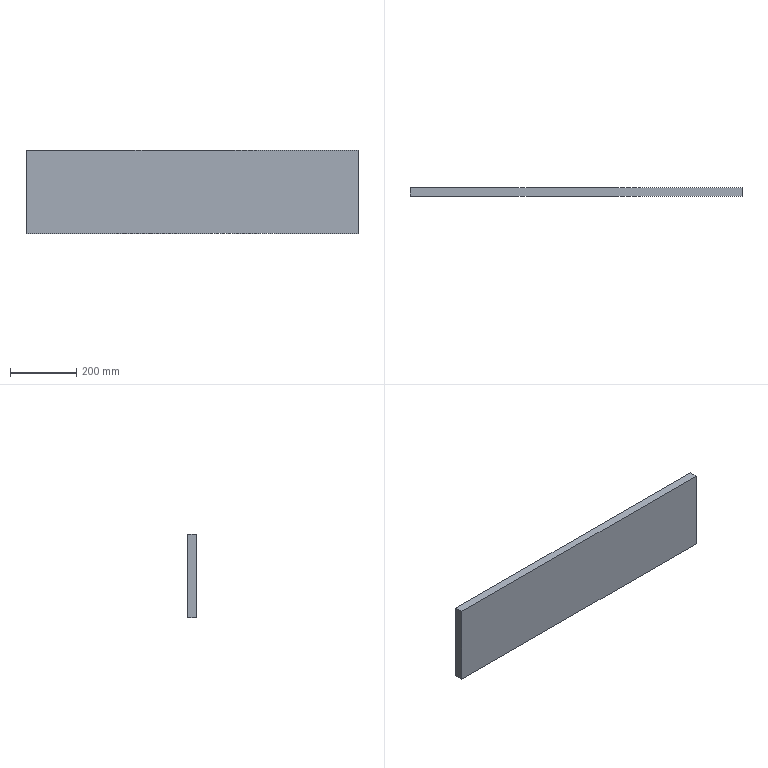Part | SolidWorks | features Fillet 3, Cut 1, Extrusion 1, LPattern 1 | 1 solid | 6 faces | box 1000 x 25 x 250 mm | volume 6250000 mm3 | plane 6
STEP:
#1=CARTESIAN_POINT('',(-500.,-12.5,-125.));
#2=VERTEX_POINT('',#1);
#3=CARTESIAN_POINT('',(-500.,-12.5,125.));
#4=VERTEX_POINT('',#3);
#5=CARTESIAN_POINT('',(-500.,-12.5,-125.));
#6=DIRECTION('',(0.,0.,1.));
#7=VECTOR('',#6,1000.);
#8=LINE('',#5,#7);
#9=EDGE_CURVE('',#2,#4,#8,.T.);
#10=ORIENTED_EDGE('',*,*,#9,.T.);
#11=CARTESIAN_POINT('',(-500.,12.5,125.));
#12=VERTEX_POINT('',#11);
#13=CARTESIAN_POINT('',(-500.,12.5,125.));
#14=DIRECTION('',(0.,-1.,0.));
#15=VECTOR('',#14,1000.);
#16=LINE('',#13,#15);
#17=EDGE_CURVE('',#12,#4,#16,.T.);
#18=ORIENTED_EDGE('',*,*,#17,.F.);
#19=CARTESIAN_POINT('',(-500.,12.5,-125.));
#20=VERTEX_POINT('',#19);
#21=CARTESIAN_POINT('',(-500.,12.5,-125.));
#22=DIRECTION('',(0.,0.,1.));
#23=VECTOR('',#22,1000.);
#24=LINE('',#21,#23);
#25=EDGE_CURVE('',#20,#12,#24,.T.);
#26=ORIENTED_EDGE('',*,*,#25,.F.);
#27=CARTESIAN_POINT('',(-500.,12.5,-125.));
#28=DIRECTION('',(0.,-1.,0.));
#29=VECTOR('',#28,1000.);
#30=LINE('',#27,#29);
#31=EDGE_CURVE('',#20,#2,#30,.T.);
#32=ORIENTED_EDGE('',*,*,#31,.T.);
#33=EDGE_LOOP('',(#10,#18,#26,#32));
#34=FACE_OUTER_BOUND('',#33,.T.);
#35=CARTESIAN_POINT('',(-500.,12.5,-125.));
#36=DIRECTION('',(1.,0.,0.));
#37=DIRECTION('',(0.,0.,-1.));
#38=AXIS2_PLACEMENT_3D('',#35,#36,#37);
#39=PLANE('',#38);
#40=ADVANCED_FACE('',(#34),#39,.F.);
#41=CARTESIAN_POINT('',(500.,-12.5,125.));
#42=VERTEX_POINT('',#41);
#43=CARTESIAN_POINT('',(-500.,-12.5,125.));
#44=DIRECTION('',(1.,0.,0.));
#45=VECTOR('',#44,1000.);
#46=LINE('',#43,#45);
#47=EDGE_CURVE('',#4,#42,#46,.T.);
#48=ORIENTED_EDGE('',*,*,#47,.T.);
#49=CARTESIAN_POINT('',(500.,12.5,125.));
#50=VERTEX_POINT('',#49);
#51=CARTESIAN_POINT('',(500.,12.5,125.));
#52=DIRECTION('',(0.,-1.,0.));
#53=VECTOR('',#52,1000.);
#54=LINE('',#51,#53);
#55=EDGE_CURVE('',#50,#42,#54,.T.);
#56=ORIENTED_EDGE('',*,*,#55,.F.);
#57=CARTESIAN_POINT('',(-500.,12.5,125.));
#58=DIRECTION('',(1.,0.,0.));
#59=VECTOR('',#58,1000.);
#60=LINE('',#57,#59);
#61=EDGE_CURVE('',#12,#50,#60,.T.);
#62=ORIENTED_EDGE('',*,*,#61,.F.);
#63=ORIENTED_EDGE('',*,*,#17,.T.);
#64=EDGE_LOOP('',(#48,#56,#62,#63));
#65=FACE_OUTER_BOUND('',#64,.T.);
#66=CARTESIAN_POINT('',(-500.,12.5,125.));
#67=DIRECTION('',(0.,0.,-1.));
#68=DIRECTION('',(-1.,0.,0.));
#69=AXIS2_PLACEMENT_3D('',#66,#67,#68);
#70=PLANE('',#69);
#71=ADVANCED_FACE('',(#65),#70,.F.);
#72=CARTESIAN_POINT('',(500.,-12.5,-125.));
#73=VERTEX_POINT('',#72);
#74=CARTESIAN_POINT('',(500.,-12.5,-125.));
#75=DIRECTION('',(0.,0.,-1.));
#76=VECTOR('',#75,1000.);
#77=LINE('',#74,#76);
#78=EDGE_CURVE('',#42,#73,#77,.T.);
#79=ORIENTED_EDGE('',*,*,#78,.T.);
#80=CARTESIAN_POINT('',(500.,12.5,-125.));
#81=VERTEX_POINT('',#80);
#82=CARTESIAN_POINT('',(500.,12.5,-125.));
#83=DIRECTION('',(0.,-1.,0.));
#84=VECTOR('',#83,1000.);
#85=LINE('',#82,#84);
#86=EDGE_CURVE('',#81,#73,#85,.T.);
#87=ORIENTED_EDGE('',*,*,#86,.F.);
#88=CARTESIAN_POINT('',(500.,12.5,-125.));
#89=DIRECTION('',(0.,0.,-1.));
#90=VECTOR('',#89,1000.);
#91=LINE('',#88,#90);
#92=EDGE_CURVE('',#50,#81,#91,.T.);
#93=ORIENTED_EDGE('',*,*,#92,.F.);
#94=ORIENTED_EDGE('',*,*,#55,.T.);
#95=EDGE_LOOP('',(#79,#87,#93,#94));
#96=FACE_OUTER_BOUND('',#95,.T.);
#97=CARTESIAN_POINT('',(500.,12.5,-125.));
#98=DIRECTION('',(-1.,0.,0.));
#99=DIRECTION('',(0.,0.,1.));
#100=AXIS2_PLACEMENT_3D('',#97,#98,#99);
#101=PLANE('',#100);
#102=ADVANCED_FACE('',(#96),#101,.F.);
#103=CARTESIAN_POINT('',(-500.,-12.5,-125.));
#104=DIRECTION('',(-1.,0.,0.));
#105=VECTOR('',#104,1000.);
#106=LINE('',#103,#105);
#107=EDGE_CURVE('',#73,#2,#106,.T.);
#108=ORIENTED_EDGE('',*,*,#107,.T.);
#109=ORIENTED_EDGE('',*,*,#31,.F.);
#110=CARTESIAN_POINT('',(-500.,12.5,-125.));
#111=DIRECTION('',(-1.,0.,0.));
#112=VECTOR('',#111,1000.);
#113=LINE('',#110,#112);
#114=EDGE_CURVE('',#81,#20,#113,.T.);
#115=ORIENTED_EDGE('',*,*,#114,.F.);
#116=ORIENTED_EDGE('',*,*,#86,.T.);
#117=EDGE_LOOP('',(#108,#109,#115,#116));
#118=FACE_OUTER_BOUND('',#117,.T.);
#119=CARTESIAN_POINT('',(-500.,12.5,-125.));
#120=DIRECTION('',(0.,0.,1.));
#121=DIRECTION('',(1.,0.,0.));
#122=AXIS2_PLACEMENT_3D('',#119,#120,#121);
#123=PLANE('',#122);
#124=ADVANCED_FACE('',(#118),#123,.F.);
#125=ORIENTED_EDGE('',*,*,#25,.T.);
#126=ORIENTED_EDGE('',*,*,#61,.T.);
#127=ORIENTED_EDGE('',*,*,#92,.T.);
#128=ORIENTED_EDGE('',*,*,#114,.T.);
#129=EDGE_LOOP('',(#125,#126,#127,#128));
#130=FACE_OUTER_BOUND('',#129,.T.);
#131=CARTESIAN_POINT('',(-500.,12.5,125.));
#132=DIRECTION('',(0.,1.,0.));
#133=DIRECTION('',(0.,0.,1.));
#134=AXIS2_PLACEMENT_3D('',#131,#132,#133);
#135=PLANE('',#134);
#136=ADVANCED_FACE('',(#130),#135,.T.);
#137=ORIENTED_EDGE('',*,*,#9,.F.);
#138=ORIENTED_EDGE('',*,*,#107,.F.);
#139=ORIENTED_EDGE('',*,*,#78,.F.);
#140=ORIENTED_EDGE('',*,*,#47,.F.);
#141=EDGE_LOOP('',(#137,#138,#139,#140));
#142=FACE_OUTER_BOUND('',#141,.T.);
#143=CARTESIAN_POINT('',(-500.,-12.5,125.));
#144=DIRECTION('',(0.,1.,0.));
#145=DIRECTION('',(0.,0.,1.));
#146=AXIS2_PLACEMENT_3D('',#143,#144,#145);
#147=PLANE('',#146);
#148=ADVANCED_FACE('',(#142),#147,.F.);
#149=CLOSED_SHELL('',(#40,#71,#102,#124,#136,#148));
#150=MANIFOLD_SOLID_BREP('',#149);
#151=CARTESIAN_POINT('',(0.,0.,0.));
#152=DIRECTION('',(0.,0.,1.));
#153=DIRECTION('',(1.,0.,0.));
#154=AXIS2_PLACEMENT_3D('',#151,#152,#153);
#155=(LENGTH_UNIT()NAMED_UNIT(*)SI_UNIT(.MILLI.,.METRE.));
#156=UNCERTAINTY_MEASURE_WITH_UNIT(LENGTH_MEASURE(0.00001),#155,'','');
#157=(NAMED_UNIT(*)PLANE_ANGLE_UNIT()SI_UNIT($,.RADIAN.));
#158=(NAMED_UNIT(*)SI_UNIT($,.STERADIAN.)SOLID_ANGLE_UNIT());
#159=(GEOMETRIC_REPRESENTATION_CONTEXT(3)GLOBAL_UNCERTAINTY_ASSIGNED_CONTEXT((#156))GLOBAL_UNIT_ASSIGNED_CONTEXT((#155,#157,#158))REPRESENTATION_CONTEXT('',''));
#160=ADVANCED_BREP_SHAPE_REPRESENTATION('',(#150,#154),#159);